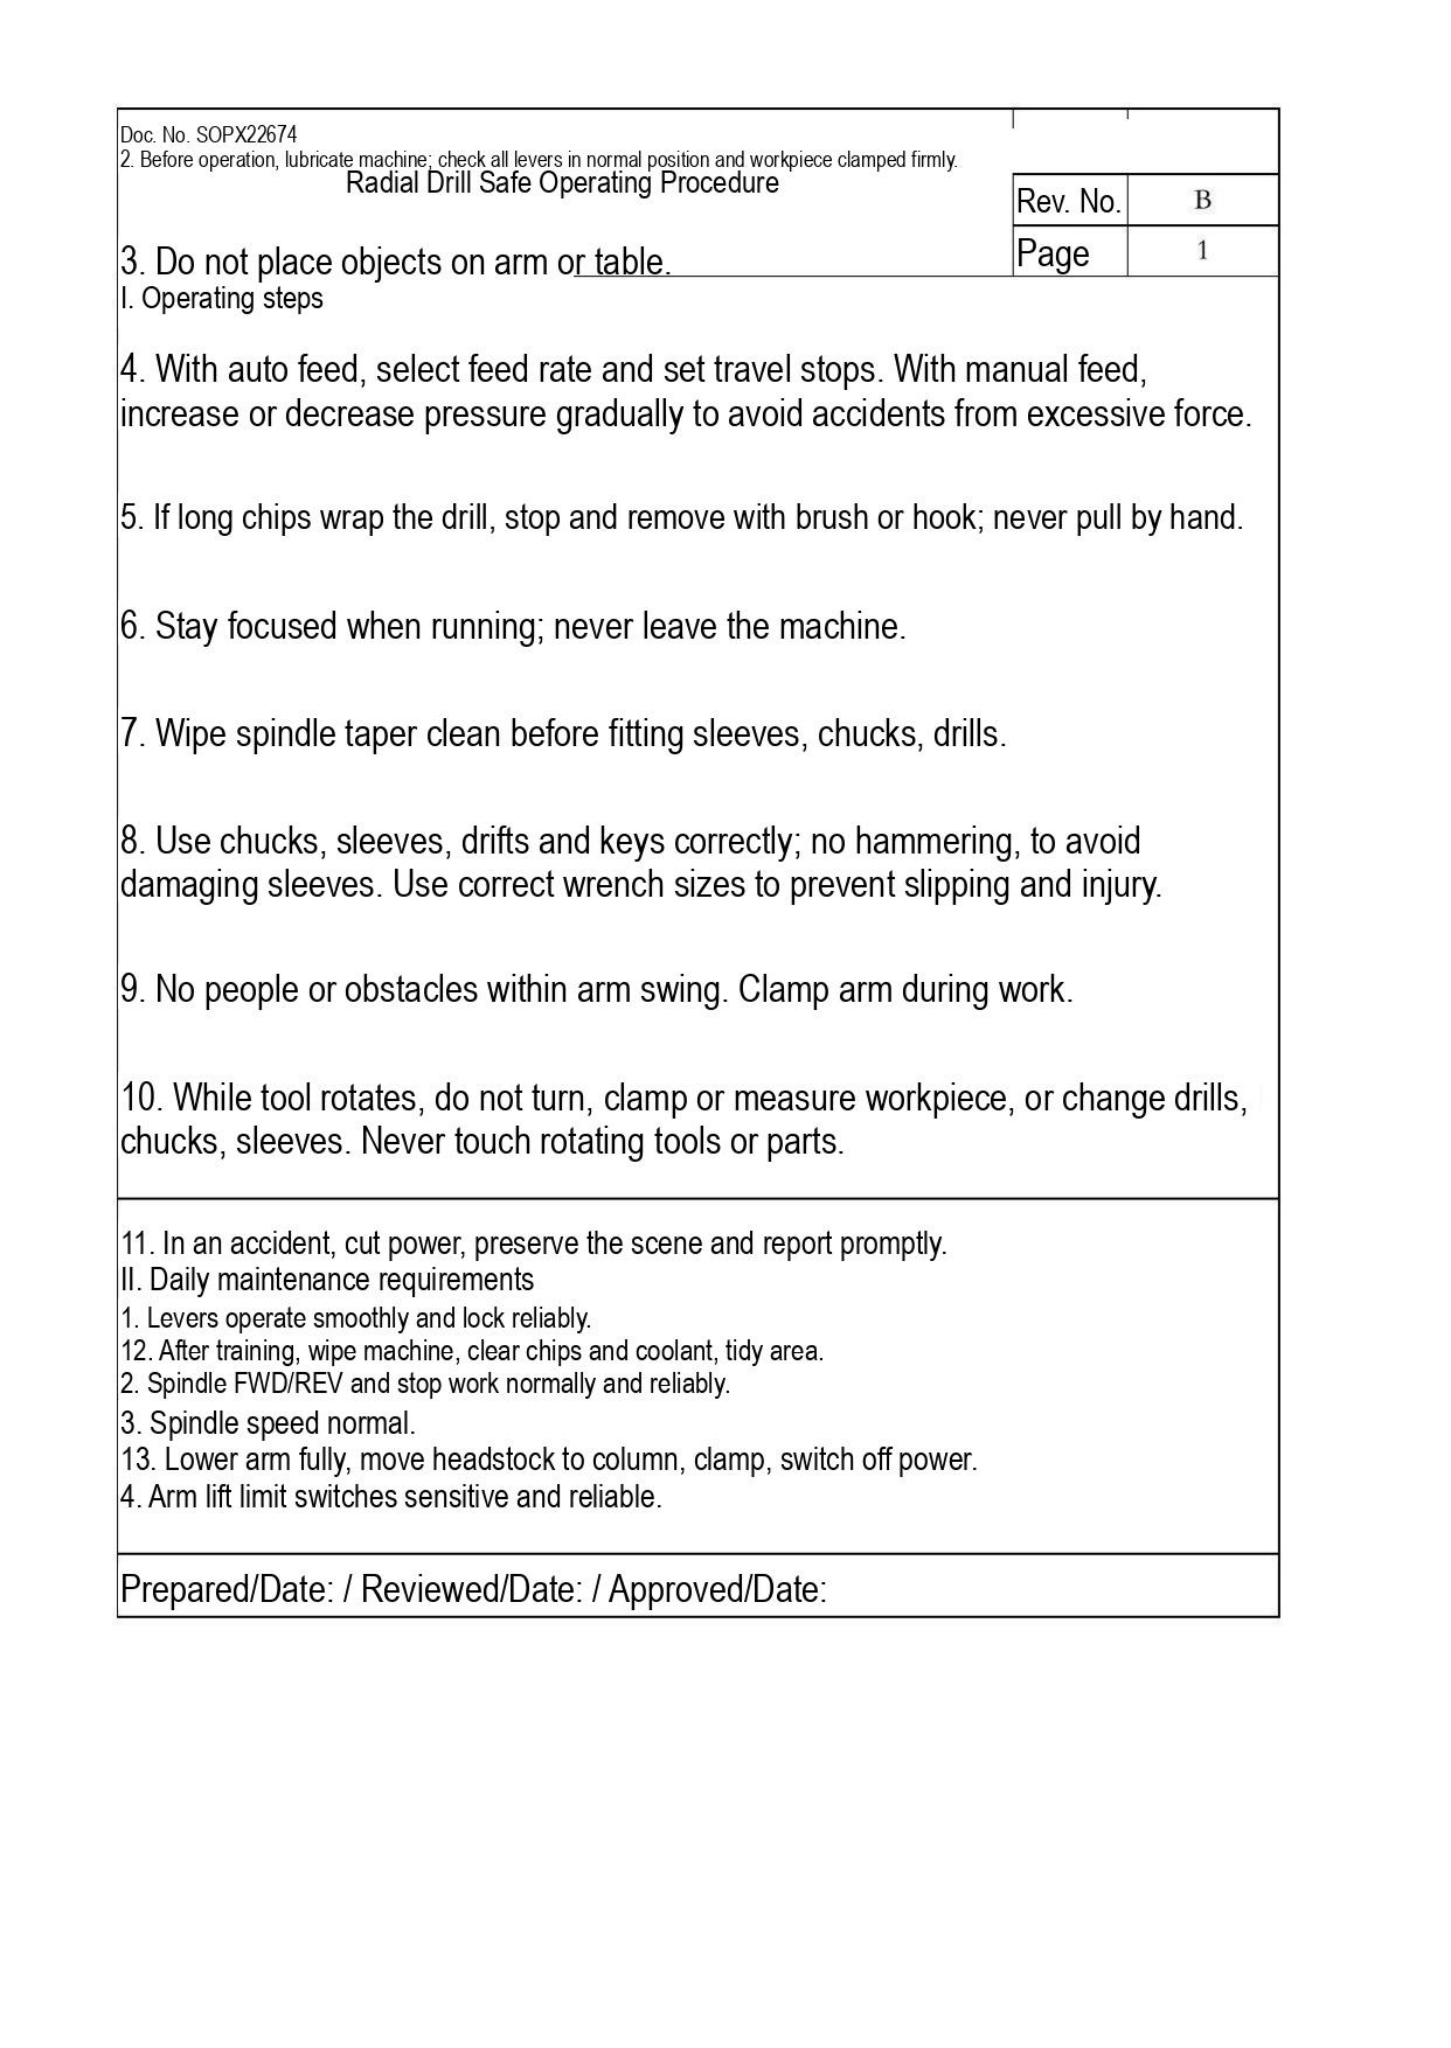Doc. No. SOPX22674
2. Before operation, lubricate machine; check all levers in normal position and workpiece clamped firmly.
Radial Drill Safe Operating Procedure

| Rev. No. | B |
|---|---|
| Page | 1 |

3. Do not place objects on arm or table.
I. Operating steps

4. With auto feed, select feed rate and set travel stops. With manual feed, increase or decrease pressure gradually to avoid accidents from excessive force.

5. If long chips wrap the drill, stop and remove with brush or hook; never pull by hand.

6. Stay focused when running; never leave the machine.

7. Wipe spindle taper clean before fitting sleeves, chucks, drills.

8. Use chucks, sleeves, drifts and keys correctly; no hammering, to avoid damaging sleeves. Use correct wrench sizes to prevent slipping and injury.

9. No people or obstacles within arm swing. Clamp arm during work.

10. While tool rotates, do not turn, clamp or measure workpiece, or change drills, chucks, sleeves. Never touch rotating tools or parts.

11. In an accident, cut power, preserve the scene and report promptly.
II. Daily maintenance requirements
1. Levers operate smoothly and lock reliably.
12. After training, wipe machine, clear chips and coolant, tidy area.
2. Spindle FWD/REV and stop work normally and reliably.
3. Spindle speed normal.
13. Lower arm fully, move headstock to column, clamp, switch off power.
4. Arm lift limit switches sensitive and reliable.

Prepared/Date: / Reviewed/Date: / Approved/Date: